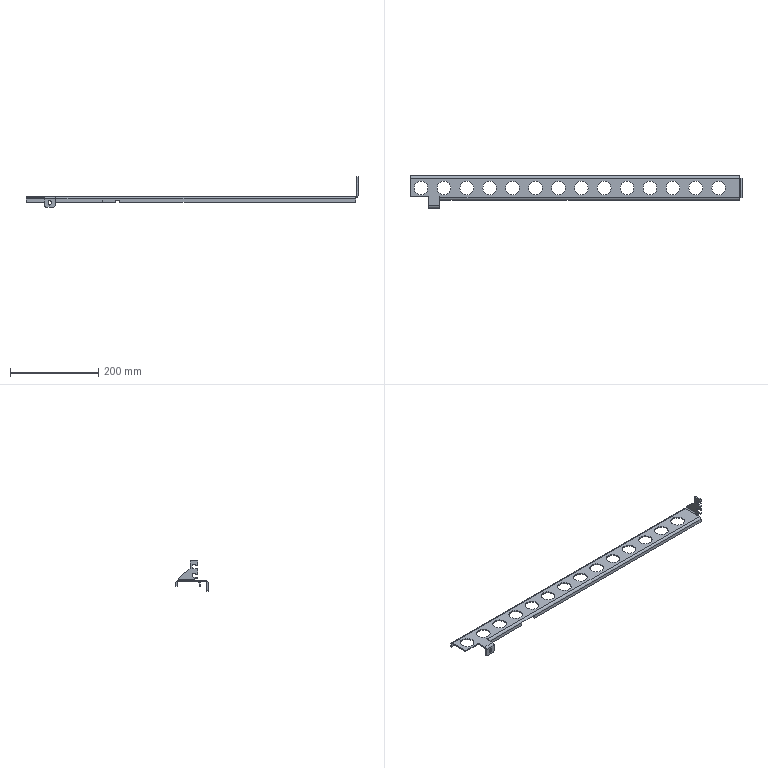Part | STEP file | 64560352 | 1 solid | 114 faces | box 754 x 73 x 68.5 mm | volume 109655 mm3 | plane 68 | cylinder 46 | commonest cylinder face diameters 31 x28 7 x6 5 x4 10 x4 8 x2 3 x1